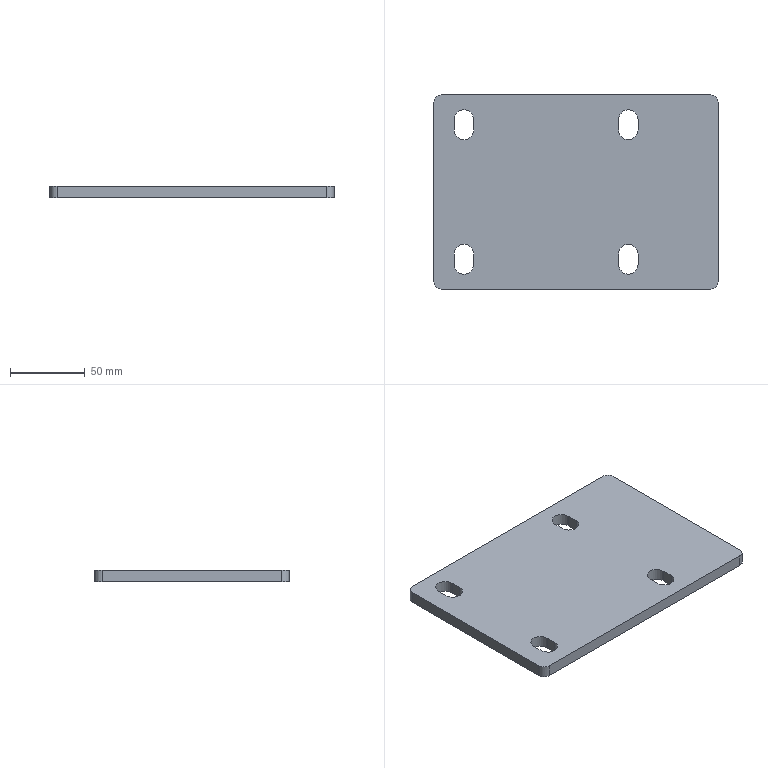Part | STEP file | HL4GD-1.30.105 cab frame front mounting plate-
-20251212 | 1 solid | 26 faces | box 190 x 130 x 8 mm | volume 190269 mm3 | plane 14 | cylinder 12 | commonest cylinder face diameters 13 x8 10 x4